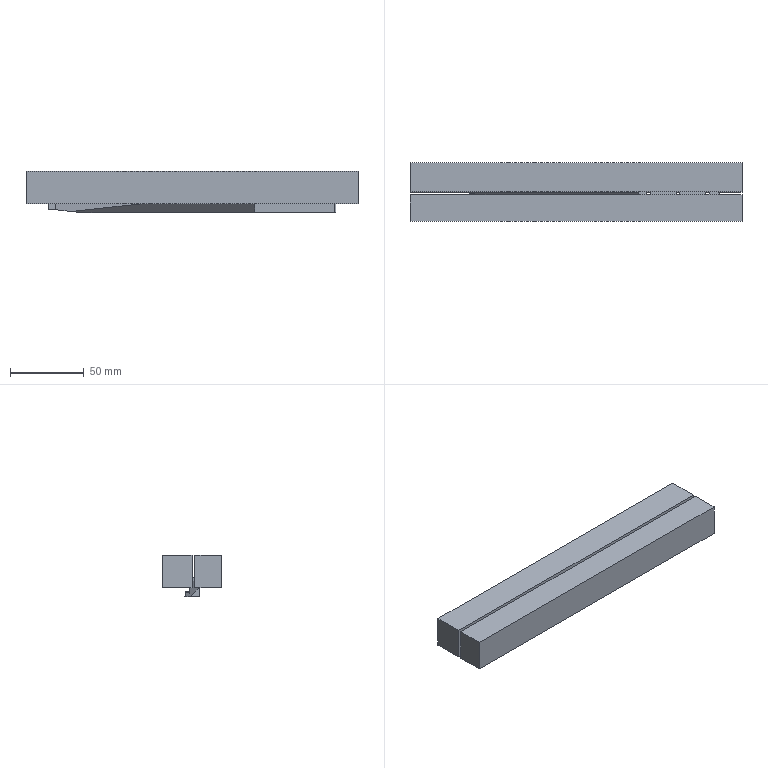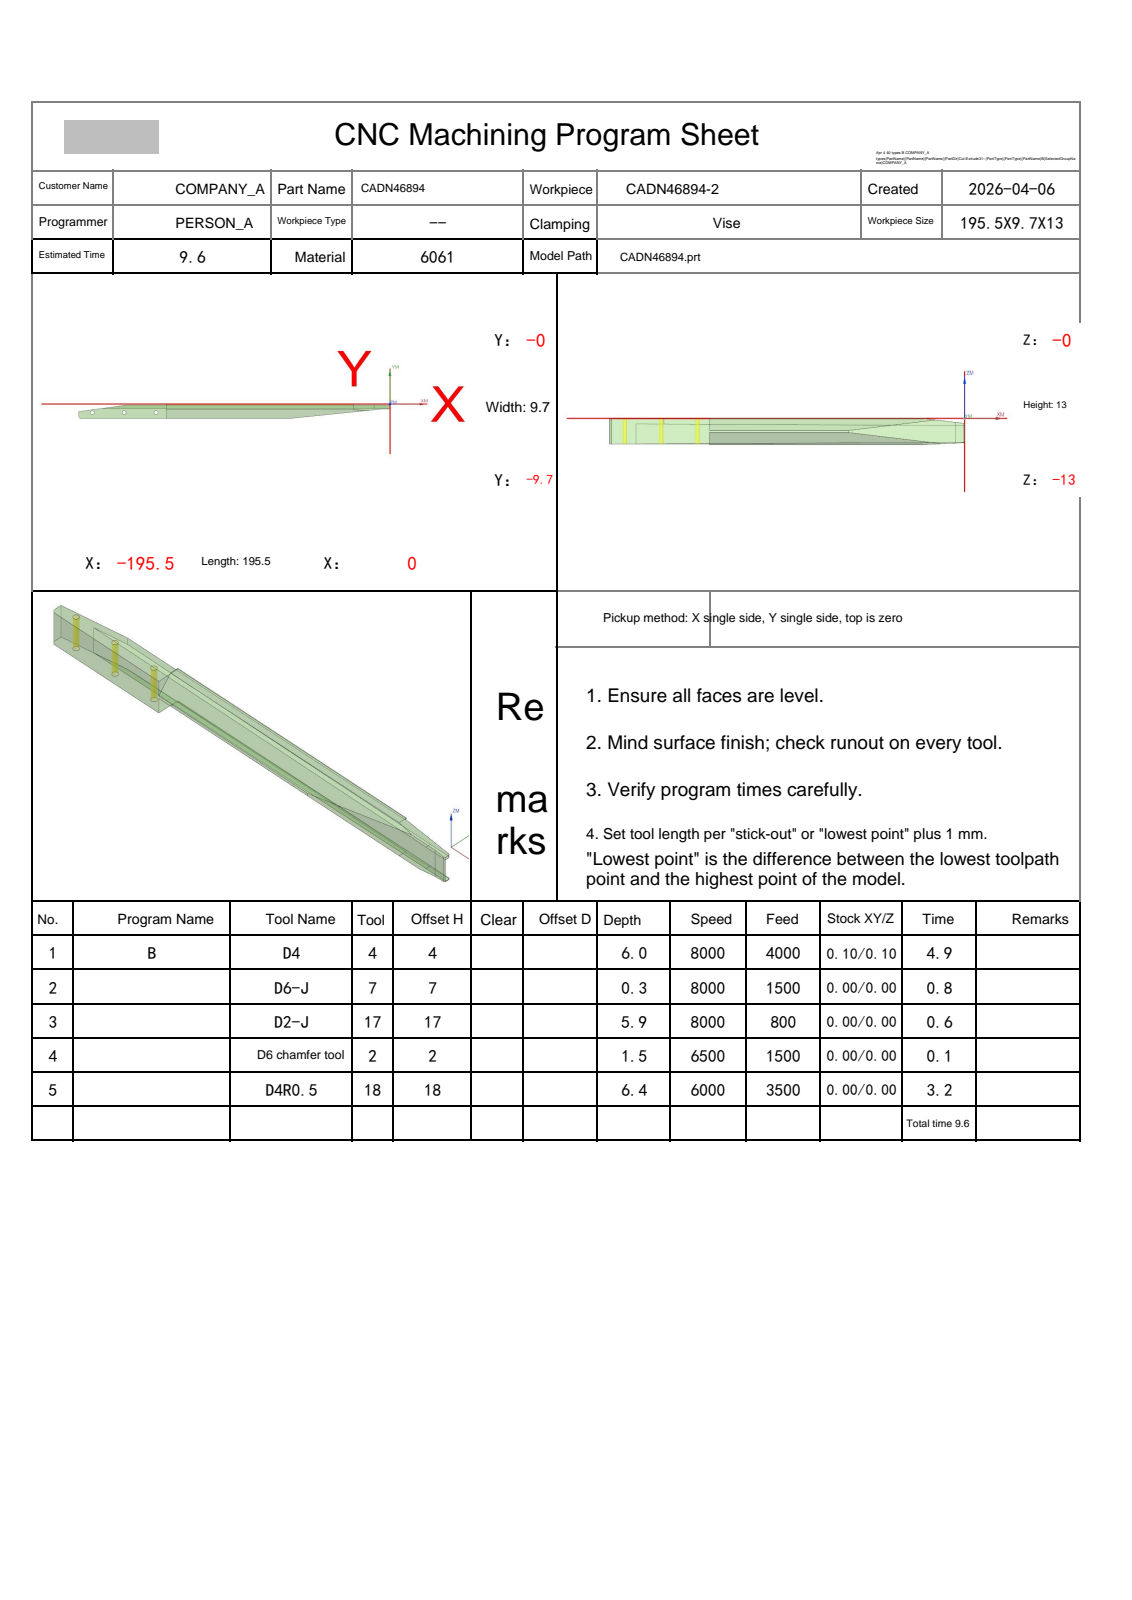NC program | NX | posted by the shop | part box 225.5 x 39.7 x 28 mm
Whole program:
%
O0001
(Machine time: 7.98 MIN)
(===Total Tool:2===)
(T4=D4      D=4.   R=0.   D-  H04 Z=-2.8  )
(T11=D4-J   D=4.   R=0.   D11 H11 Z=-2.9  )
G80 G90 G17 G49 G40
G91 G28 Z0
M01
N1 T04 M06
(D4  D=4. R=0. H=04 ce=0.10 di=0.10)
G00 G90 G54 X-16.475 Y1.3 M03 S8000
G43 H04 Z50.
M08
Z.576
G01 X-40.723 Z-.059 F2000.
Y0.0 Z-.093
X-40.722 Y-1.3
X72.723
Y1.3
X-40.723
Y0.0
X-43.523 Y-.001
X-43.521 Y-4.201
X-43.42 Y-4.1
X75.523
Y4.1
X-43.42
X-43.525 Y4.205
X-43.524 Y3.595
X-43.523 Y-.001
X-43.522 Y-.501
Z.407
G00 Z.576
X-15.143 Y.583
Z.407
G01 X-40.017 Y.687 Z-.244
X-40.015 Y.013 Z-.262
X-40.014 Y-.671
X72.002 Y-.216
Y.216
X-40.017 Y.687
X-40.015 Y.013
X-41.815 Y.01
X-41.811 Y-2.479
X73.802 Y-2.009
Y2.009
X-41.82 Y2.495
X-41.815 Y.01
X-43.915 Y.006
Y-1.237
X-43.907 Y-4.587
X-43.42 Y-4.1
X75.902
Y4.1
X-43.42
X-43.924 Y4.604
X-43.915 Y.006
Y-.494
Z.238
G00 Z.407
X-17.378 Y1.3
Z.238
G01 X-41.627 Z-.397
Y0.0 Z-.431
Y-1.3
X73.624
Y1.3
X-41.627
Y0.0
X-44.427
X-44.429 Y-5.11
X-43.42 Y-4.1
X76.424
Y4.1
X-43.42
X-44.427 Y5.107
Y0.0
Y-.5
Z.069
G00 Z.238
X-18.259 Y1.3
Z.069
G01 X-42.508 Z-.566
X-42.518 Y0.0 Z-.6
X-42.527 Y-1.3
X74.52
X74.524 Y1.3
X-42.508
X-42.518 Y0.0
X-45.317 Y.021
X-45.354 Y-6.6
X-44.85
Y-5.53
X-43.42 Y-4.1
X76.85
Y-6.677
X77.315 Y-6.626
X77.332 Y6.8
X76.85 Y6.819
Y4.1
X-43.42
X-44.85 Y5.53
Y6.6
X-45.267
X-45.317 Y.021
X-45.321 Y-.479
Z-.1
G00 Z.069
X-73.548 Y1.2
Z-.3
G01 Z-.8
X-67.047
Y.232
X87.742 Y.9
X96.104
Y1.5
X87.742
X-67.047 Y2.168
Y1.2
X-68.847
Y-1.575
X87.745 Y-.9
X97.904
Y3.3
X87.745
X-68.847 Y3.975
Y1.2
Y.7
Z-.3
G00 Z-.1
X-74.943 Y1.2
Z-.5
G01 Z-1.
X-68.442
Y.226
X87.742 Y.9
X96.324
Y1.5
X87.742
X-68.442 Y2.174
Y1.2
X-70.242
Y-1.581
X87.745 Y-.9
X98.124
Y3.3
X87.745
X-70.241 Y3.981
X-70.242 Y1.2
Y.7
Z-.5
G00 Z-.3
X-76.338 Y1.2
Z-.7
G01 Z-1.2
X-69.835
Y.22
X87.742 Y.9
X96.331
Y1.5
X87.742
X-69.835 Y2.18
Y1.2
X-71.635
Y-1.587
X87.745 Y-.9
X98.131
Y3.3
X87.745
X-71.635 Y3.987
Y1.2
Y.7
Z-.7
G00 Z-.5
X-77.734 Y1.2
Z-.9
G01 Z-1.4
X-71.23
Y.214
X87.742 Y.9
X96.338
Y1.5
X87.742
X-71.23 Y2.186
Y1.2
X-73.03
X-73.031 Y-1.593
X87.745 Y-.9
X98.138
Y3.3
X87.745
X-73.03 Y3.993
Y1.2
Y.7
Z-.9
G00 Z-.7
X-79.129 Y1.2
Z-1.1
G01 Z-1.6
X-72.624
Y.208
X87.742 Y.9
X96.343
Y1.5
X87.742
X-72.624 Y2.192
Y1.2
X-74.424
Y-1.599
X87.745 Y-.9
X98.143
Y3.3
X87.745
X-74.424 Y3.999
Y1.2
Y.7
Z-1.1
G00 Z-.9
X-80.524 Y1.2
Z-1.3
G01 Z-1.8
X-74.018
X-74.019 Y.202
X87.742 Y.9
X96.348
Y1.5
X87.742
X-74.018 Y2.198
Y1.2
X-75.818
X-75.819 Y-1.175
Y-1.605
X87.745 Y-.9
X98.148
Y3.3
X87.745
X-75.818 Y4.005
Y1.2
X-75.819 Y.7
Z-1.3
G00 Z-1.1
X-81.92 Y1.2
Z-1.5
G01 Z-2.
X-75.413
Y.196
X87.742 Y.9
X96.349
Y1.5
X87.742
X-75.413 Y2.204
Y1.2
X-77.213
Y-.199
X-77.215 Y-1.611
X87.745 Y-.9
X98.149
Y3.3
X87.745
X-77.212 Y4.011
X-77.213 Y1.2
Y.7
Z-1.5
G00 Z-1.3
X-54.691 Y3.914
Z-1.5
G01 X-78.607 Y4.017 Z-2.126
X-78.608 Y1.201 Z-2.2
X-75.808 Y1.2
Y1.195
X-74.573 Y1.2
X-72.573
G03 X-72.737 Y1.992 I-2. J0.0
G01 X87.745 Y1.3
X96.149
Y1.1
X87.737
X-72.737 Y.408
G03 X-72.573 Y1.2 I-1.836 J.792
G01 X-74.573
X-75.808 Y1.205
Y1.2
X-78.608 Y1.201
X-78.609 Y-1.074
X-78.61 Y-1.617
X87.745 Y-.9
X98.149
Y3.3
X87.745
X-78.607 Y4.017
X-78.608 Y1.201
X-78.609 Y.701
Z-1.7
G00 Z-1.5
X-56.092 Y3.92
Z-1.7
G01 X-80.001 Y4.023 Z-2.326
X-80.003 Y1.202 Z-2.4
X-77.203 Y1.2
Y1.189
X-74.573 Y1.2
X-72.573
G03 X-72.737 Y1.992 I-2. J0.0
G01 X87.745 Y1.3
X96.148
Y1.1
X87.737
X-72.737 Y.408
G03 X-72.573 Y1.2 I-1.836 J.792
G01 X-74.573
X-77.203 Y1.211
Y1.2
X-80.003 Y1.202
X-80.004 Y-.199
X-80.005 Y-1.623
X87.745 Y-.9
X98.148
Y3.3
X87.745
X-80.001 Y4.023
X-80.003 Y1.202
Y.702
Z-1.9
G00 Z-1.7
X-76.145 Y1.207
Z-1.9
G01 X-78.599 Y1.217 Z-1.964
Y1.183 Z-1.965
X-74.573 Y1.2 Z-2.071
X-78.599 Y1.217 Z-2.176
Y1.183 Z-2.177
X-74.573 Y1.2 Z-2.282
X-78.599 Y1.217 Z-2.388
Y1.183 Z-2.389
X-74.573 Y1.2 Z-2.494
X-78.599 Y1.217 Z-2.6
Y1.2
Y1.183
X-74.573 Y1.2
X-72.573
G03 X-72.737 Y1.992 I-2. J0.0
G01 X87.745 Y1.3
X96.145
Y1.1
X87.737
X-72.737 Y.408
G03 X-72.573 Y1.2 I-1.836 J.792
G01 X-74.573
X-78.599 Y1.217
Y1.2
X-81.399 Y1.202
X-81.401 Y-1.629
X87.745 Y-.9
X98.145
Y3.3
X87.745
X-81.397 Y4.029
X-81.399 Y1.202
Y.702
Z-2.1
G00 Z-1.9
X-75.026 Y1.202
Z-2.1
G01 X-79.987 Y1.223 Z-2.23
Y1.177 Z-2.231
X-74.573 Y1.2 Z-2.373
X-79.987 Y1.223 Z-2.515
Y1.177 Z-2.516
X-74.573 Y1.2 Z-2.658
X-79.987 Y1.223 Z-2.799
Y1.2 Z-2.8
Y1.177
X-74.573 Y1.2
X-72.573
G03 X-72.737 Y1.992 I-2. J0.0
G01 X87.745 Y1.3
X96.14
X96.141 Y1.1
X87.737
X-72.737 Y.408
G03 X-72.573 Y1.2 I-1.836 J.792
G01 X-74.573
X-79.987 Y1.223
Y1.2
X-82.787 Y1.202
Y-.199
X-82.789 Y-1.635
X87.745 Y-.9
X98.141
X98.14 Y2.263
X98.139 Y3.3
X87.745
X-82.785 Y4.035
X-82.787 Y1.202
Y.702
Z-2.3
G00 Z50.
G91 G28 Z0.0
M05
M09
G91 G28 Z0.0
M01
N2 T11 M06
(D4-J  D=4. R=0. H=11 ce=0.40 di=0.00)
G00 G90 G54 X-58.552 Y9. M03 S7000
G43 H11 Z12.2
M08
Z.8
G01 Z-.7 F1000.
Y7.4
G03 X-57.752 Y6.6 I.8 J0.0
G01 X-46.507
G02 X-46.229 Y6.485 I-.003 J-.4
G01 X-43.544 Y3.8
X77.15
Y6.435
G02 X77.51 Y6.792 I.36 J-.003
G01 X77.521
X97.312 Y6.017
G02 X97.65 Y5.8 I-.018 J-.4
G01 X97.743
G02 X98.14 Y5.403 I-.003 J-.4
G01 Y-3.003
G02 X97.743 Y-3.4 I-.4 J.003
G01 X97.65
Y-4.057
G02 X97.296 Y-4.452 I-.4 J.003
G01 X77.502 Y-6.603
X77.47 Y-6.605
G02 X77.15 Y-6.287 I0.0 J.32
G01 Y-3.8
X-43.544
X-46.229 Y-6.485
G02 X-46.507 Y-6.6 I-.281 J.285
G01 X-67.814
G02 X-68.15 Y-6.413 I.003 J.4
G01 X-71.599 Y-4.087
X-83.14 Y-4.137
G02 X-83.499 Y-3.78 I.001 J.36
G01 Y6.18
G02 X-83.14 Y6.537 I.36 J-.003
G01 X-81.499 Y6.53
X-68.15 Y6.472
G02 X-67.86 Y6.6 I.293 J-.272
G01 X-56.918
G02 X-56.635 Y6.483 I0.0 J-.4
G01 X-54.869 Y4.717
G03 X-54.587 Y4.6 I.283 J.283
G01 X-47.335
G02 X-47.058 Y4.485 I-.003 J-.4
G01 X-44.958 Y2.386
G03 X-43.544 Y1.8 I1.414 J1.414
G01 X77.15
G03 X79.15 Y3.8 I0.0 J2.
G01 Y4.314
G02 X79.55 Y4.711 I.4 J-.003
G01 X79.562 Y4.71
X95.759 Y4.077
G02 X96.14 Y3.68 I-.019 J-.4
G01 Y-1.95
G02 X96.06 Y-2.187 I-.4 J.003
G03 X95.904 Y-2.425 I1.59 J-1.213
G02 X95.603 Y-2.624 I-.347 J.198
G01 X79.59 Y-4.364
X79.55 Y-4.366
G02 X79.15 Y-3.97 I0.0 J.4
G01 Y-3.8
G03 X78.921 Y-2.871 I-2. J0.0
G01 X78.875 Y-2.685
X78.878 Y-2.636
X79.138 Y-.546
X79.141 Y-.497
G03 X79.055 Y-.249 I-.4 J0.0
G02 X78.968 Y0.0 I.313 J.249
X79.164 Y.344 I.4 J0.0
G03 X80.892 Y2.387 I-2.014 J3.456
G02 X81.265 Y2.642 I.373 J-.145
G01 X81.277
X93.759 Y2.153
G02 X94.14 Y1.757 I-.019 J-.4
G01 Y-.416
G02 X93.787 Y-.81 I-.4 J.003
G01 X81.104 Y-2.188
X81.064 Y-2.19
G02 X80.71 Y-1.976 I0.0 J.4
G03 X80.204 Y-1.217 I-3.56 J-1.824
G02 X80.129 Y-1.011 I.244 J.207
X80.274 Y-.742 I.32 J0.0
G01 X82.092 Y.441
X82.139 Y.463
X82.169 Y.506
G02 X82.376 Y.597 I.207 J-.189
G01 X82.384
X85.593 Y.471
X85.669 Y.392
X85.599 Y.312
X82.932 Y.022
X82.927
X79.274 Y-.333
G03 X79.074 Y-.41 I.039 J-.398
G01 X77.312 Y-1.721
G02 X77.074 Y-1.8 I-.238 J.321
G01 X-43.544
G03 X-44.958 Y-2.386 I0.0 J-2.
G01 X-47.058 Y-4.485
G02 X-47.335 Y-4.6 I-.281 J.285
G01 X-67.142
G02 X-67.36 Y-4.534 I.003 J.4
G01 X-70.481 Y-2.429
G03 X-71.599 Y-2.087 I-1.118 J-1.658
G01 X-71.608
X-81.1 Y-2.128
G02 X-81.499 Y-1.731 I.002 J.4
G01 Y4.131
G02 X-81.1 Y4.528 I.4 J-.003
G01 X-68.159 Y4.472
X-68.15
G03 X-67.504 Y4.58 I0.0 J2.
G01 X-67.445 Y4.605
X-67.381 Y4.6
X-56.918
G02 X-56.635 Y4.483 I0.0 J-.4
G01 X-54.869 Y2.717
G03 X-54.587 Y2.6 I.283 J.283
G01 X-48.163
G02 X-47.886 Y2.485 I-.003 J-.4
G01 X-46.373 Y.972
G03 X-45.558 Y.344 I2.828 J2.828
G02 X-45.362 Y0.0 I-.205 J-.344
X-45.558 Y-.344 I-.4 J0.0
G03 X-46.373 Y-.972 I2.014 J-3.456
G01 X-47.886 Y-2.485
G02 X-48.163 Y-2.6 I-.28 J.285
G01 X-66.531
G02 X-66.748 Y-2.534 I.003 J.4
G01 X-69.363 Y-.771
G03 X-71.599 Y-.087 I-2.236 J-3.317
G01 X-71.617
X-79.101 Y-.12
G02 X-79.499 Y.277 I.002 J.4
G01 Y2.123
G02 X-79.101 Y2.52 I.4 J-.003
G01 X-68.167 Y2.472
X-68.15
G03 X-67.19 Y2.589 I0.0 J4.
G01 X-67.147 Y2.607
X-67.101 Y2.6
X-56.918
G02 X-56.635 Y2.483 I0.0 J-.4
G01 X-54.869 Y.717
G03 X-54.587 Y.6 I.283 J.283
G01 X-48.991
G02 X-48.715 Y.485 I-.004 J-.4
G01 X-48.51 Y.28
G02 X-48.395 Y0.0 I-.285 J-.28
X-48.51 Y-.28 I-.4 J0.0
G01 X-48.715 Y-.485
G02 X-48.991 Y-.6 I-.28 J.285
G01 X-65.92
G02 X-66.137 Y-.534 I.004 J.4
G01 X-66.736 Y-.13
G02 X-66.91 Y.2 I.227 J.33
X-66.513 Y.6 I.4 J0.0
G01 X-55.752
X-54.752
G03 X-53.952 Y1.4 I0.0 J.8
G01 Z.8
G00 Z12.2
X-85.899 Y.4
Z-1.4
G01 Z-2.9
X-84.299
G03 X-83.499 Y1.2 I0.0 J.8
G01 Y3.379
G02 X-83.14 Y3.737 I.36 J-.002
G01 X42.33 Y3.196
G02 X42.726 Y2.836 I-.002 J-.4
G01 X42.784 Y2.267
G03 X42.937 Y1.991 I.398 J.041
G02 X43.326 Y1.2 I-.612 J-.791
X42.326 Y.2 I-1. J0.0
G01 X23.937
G02 X22.937 Y1.2 I0.0 J1.
X23.937 Y2.2 I1. J0.0
G01 X41.487
G03 X41.882 Y2.537 I0.0 J.4
G01 X41.933 Y2.859
G02 X42.328 Y3.196 I.395 J-.063
G01 X42.33
X87.745 Y3.
X97.742
G02 X98.14 Y2.602 I-.002 J-.4
G01 Y-.202
G02 X97.742 Y-.6 I-.4 J.002
G01 X87.745
X-83.14 Y-1.337
G02 X-83.499 Y-.979 I.001 J.36
G01 Y3.2
G02 X-83.099 Y3.6 I.4 J0.0
X-82.859 Y3.52 I0.0 J-.4
G01 X-80.568 Y1.804
G03 X-80.33 Y1.725 I.239 J.32
G01 X22.819 Y1.28
X22.897 Y1.2
X22.819 Y1.12
X-81.1 Y.672
G02 X-81.499 Y1.069 I.001 J.4
G01 Y1.331
G02 X-81.414 Y1.574 I.4 J-.003
X-81.1 Y1.728 I.315 J-.246
G01 X-80.462 Y1.725
X-80.459
G03 X-79.659 Y2.522 I0.0 J.8
G01 Z-1.4
G00 Z12.2
G00 G90 X-46.045 Y-8.948 M03 S6000
Z50.
Z1.31
G01 Z-.69 F800.
G41 D11
X-45.75 Y-9.
G03 X-44.75 Y-8. I0.0 J1.
G01 Y-5.572
X-43.378 Y-4.2
X76.75
Y-8.096
G03 X77.75 Y-9.096 I1. J0.0
G01 G40 X78.045 Y-9.044
Z1.31
G00 Z50.
Y9.171
Z1.31
G01 Z-.69
G41 D11
X77.75 Y9.223
G03 X76.75 Y8.223 I0.0 J-1.
G01 Y4.2
X-43.378
X-44.75 Y5.572
Y8.
G03 X-45.75 Y9. I-1. J0.0
G01 G40 X-46.045 Y8.948
Z1.31
G00 Z50.
X-85.771 Y-.453
Z-.89
G01 Z-2.89
G41 D11
X-85.822 Y-.749
G03 X-84.822 Y-1.744 I1. J.004
G01 X-84.817
X87.746 Y-1.
X99.491
G03 X100.491 Y0.0 I0.0 J1.
G01 G40 X100.438 Y.295
Y2.105
G41 D11
X100.49 Y2.4
G03 X99.49 Y3.4 I-1. J0.0
G01 X87.746
X-84.813 Y4.144
X-84.817
G03 X-85.817 Y3.149 I0.0 J-1.
G01 G40 X-85.766 Y2.853
Z-.89
G00 Z50.
M05
M09
G91 G28 Z0.0
G91 G28 Y0.0
M30
%